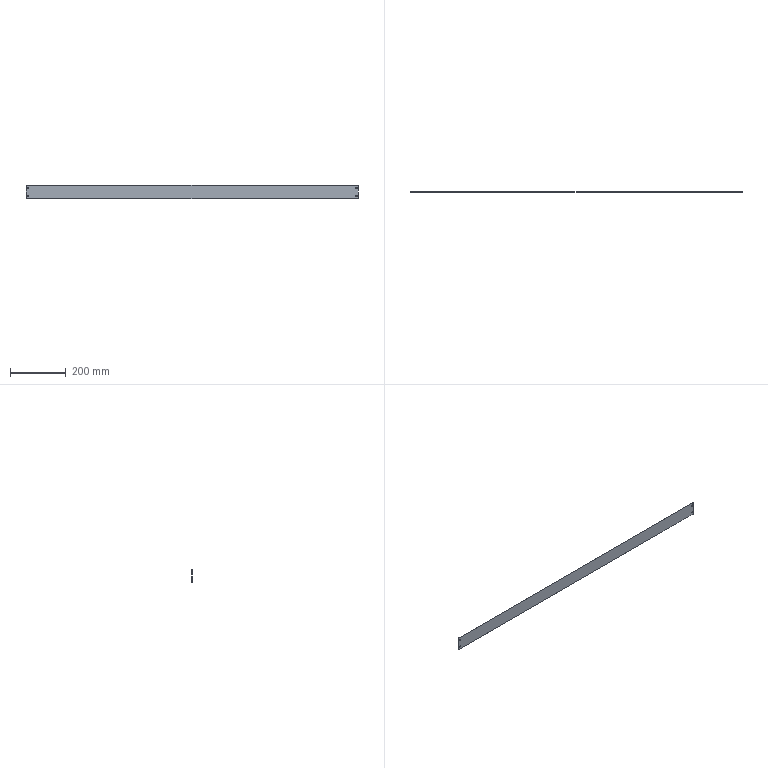Part | NX | features BREP 1 | 1 solid | 26 faces | box 1190 x 0.2 x 50 mm | volume 11880 mm3 | plane 14 | cylinder 12 | commonest cylinder face diameters 4 x12
STEP:
#1=CARTESIAN_POINT('',(591.,0.2,-16.5));
#2=VERTEX_POINT('',#1);
#3=CARTESIAN_POINT('',(588.,0.2,-16.5));
#4=VERTEX_POINT('',#3);
#5=CARTESIAN_POINT('',(591.,0.2,-16.5));
#6=DIRECTION('',(-1.,0.,0.));
#7=VECTOR('',#6,1000.);
#8=LINE('',#5,#7);
#9=EDGE_CURVE('',#2,#4,#8,.T.);
#10=ORIENTED_EDGE('',*,*,#9,.T.);
#11=CARTESIAN_POINT('',(588.,0.,-16.5));
#12=VERTEX_POINT('',#11);
#13=CARTESIAN_POINT('',(588.,0.,-16.5));
#14=DIRECTION('',(0.,1.,0.));
#15=VECTOR('',#14,1000.);
#16=LINE('',#13,#15);
#17=EDGE_CURVE('',#12,#4,#16,.T.);
#18=ORIENTED_EDGE('',*,*,#17,.F.);
#19=CARTESIAN_POINT('',(591.,0.,-16.5));
#20=VERTEX_POINT('',#19);
#21=CARTESIAN_POINT('',(591.,0.,-16.5));
#22=DIRECTION('',(-1.,0.,0.));
#23=VECTOR('',#22,1000.);
#24=LINE('',#21,#23);
#25=EDGE_CURVE('',#20,#12,#24,.T.);
#26=ORIENTED_EDGE('',*,*,#25,.F.);
#27=CARTESIAN_POINT('',(591.,0.,-16.5));
#28=DIRECTION('',(0.,1.,0.));
#29=VECTOR('',#28,1000.);
#30=LINE('',#27,#29);
#31=EDGE_CURVE('',#20,#2,#30,.T.);
#32=ORIENTED_EDGE('',*,*,#31,.T.);
#33=EDGE_LOOP('',(#10,#18,#26,#32));
#34=FACE_BOUND('',#33,.T.);
#35=CARTESIAN_POINT('',(591.,0.,-16.5));
#36=DIRECTION('',(0.,0.,-1.));
#37=DIRECTION('',(-1.,0.,0.));
#38=AXIS2_PLACEMENT_3D('',#35,#36,#37);
#39=PLANE('',#38);
#40=ADVANCED_FACE('',(#34),#39,.F.);
#41=CARTESIAN_POINT('',(588.,0.2,-12.5));
#42=VERTEX_POINT('',#41);
#43=CARTESIAN_POINT('',(588.,0.2,-14.5));
#44=DIRECTION('',(0.,1.,0.));
#45=DIRECTION('',(0.,0.,-1.));
#46=AXIS2_PLACEMENT_3D('',#43,#44,#45);
#47=CIRCLE('',#46,2.);
#48=EDGE_CURVE('',#4,#42,#47,.T.);
#49=ORIENTED_EDGE('',*,*,#48,.T.);
#50=CARTESIAN_POINT('',(588.,0.,-12.5));
#51=VERTEX_POINT('',#50);
#52=CARTESIAN_POINT('',(588.,0.,-12.5));
#53=DIRECTION('',(0.,1.,0.));
#54=VECTOR('',#53,1000.);
#55=LINE('',#52,#54);
#56=EDGE_CURVE('',#51,#42,#55,.T.);
#57=ORIENTED_EDGE('',*,*,#56,.F.);
#58=CARTESIAN_POINT('',(588.,0.,-14.5));
#59=DIRECTION('',(0.,1.,0.));
#60=DIRECTION('',(0.,0.,-1.));
#61=AXIS2_PLACEMENT_3D('',#58,#59,#60);
#62=CIRCLE('',#61,2.);
#63=EDGE_CURVE('',#12,#51,#62,.T.);
#64=ORIENTED_EDGE('',*,*,#63,.F.);
#65=ORIENTED_EDGE('',*,*,#17,.T.);
#66=EDGE_LOOP('',(#49,#57,#64,#65));
#67=FACE_BOUND('',#66,.T.);
#68=CARTESIAN_POINT('',(588.,0.,-14.5));
#69=DIRECTION('',(0.,1.,0.));
#70=DIRECTION('',(0.,0.,1.));
#71=AXIS2_PLACEMENT_3D('',#68,#69,#70);
#72=CYLINDRICAL_SURFACE('',#71,2.);
#73=ADVANCED_FACE('',(#67),#72,.F.);
#74=CARTESIAN_POINT('',(591.,0.2,-12.5));
#75=VERTEX_POINT('',#74);
#76=CARTESIAN_POINT('',(591.,0.2,-12.5));
#77=DIRECTION('',(1.,0.,0.));
#78=VECTOR('',#77,1000.);
#79=LINE('',#76,#78);
#80=EDGE_CURVE('',#42,#75,#79,.T.);
#81=ORIENTED_EDGE('',*,*,#80,.T.);
#82=CARTESIAN_POINT('',(591.,0.,-12.5));
#83=VERTEX_POINT('',#82);
#84=CARTESIAN_POINT('',(591.,0.,-12.5));
#85=DIRECTION('',(0.,1.,0.));
#86=VECTOR('',#85,1000.);
#87=LINE('',#84,#86);
#88=EDGE_CURVE('',#83,#75,#87,.T.);
#89=ORIENTED_EDGE('',*,*,#88,.F.);
#90=CARTESIAN_POINT('',(591.,0.,-12.5));
#91=DIRECTION('',(1.,0.,0.));
#92=VECTOR('',#91,1000.);
#93=LINE('',#90,#92);
#94=EDGE_CURVE('',#51,#83,#93,.T.);
#95=ORIENTED_EDGE('',*,*,#94,.F.);
#96=ORIENTED_EDGE('',*,*,#56,.T.);
#97=EDGE_LOOP('',(#81,#89,#95,#96));
#98=FACE_BOUND('',#97,.T.);
#99=CARTESIAN_POINT('',(591.,0.,-12.5));
#100=DIRECTION('',(0.,0.,1.));
#101=DIRECTION('',(1.,0.,0.));
#102=AXIS2_PLACEMENT_3D('',#99,#100,#101);
#103=PLANE('',#102);
#104=ADVANCED_FACE('',(#98),#103,.F.);
#105=CARTESIAN_POINT('',(591.,0.2,-14.5));
#106=DIRECTION('',(0.,1.,0.));
#107=DIRECTION('',(0.,0.,-1.));
#108=AXIS2_PLACEMENT_3D('',#105,#106,#107);
#109=CIRCLE('',#108,2.);
#110=EDGE_CURVE('',#75,#2,#109,.T.);
#111=ORIENTED_EDGE('',*,*,#110,.T.);
#112=ORIENTED_EDGE('',*,*,#31,.F.);
#113=CARTESIAN_POINT('',(591.,0.,-14.5));
#114=DIRECTION('',(0.,1.,0.));
#115=DIRECTION('',(0.,0.,-1.));
#116=AXIS2_PLACEMENT_3D('',#113,#114,#115);
#117=CIRCLE('',#116,2.);
#118=EDGE_CURVE('',#83,#20,#117,.T.);
#119=ORIENTED_EDGE('',*,*,#118,.F.);
#120=ORIENTED_EDGE('',*,*,#88,.T.);
#121=EDGE_LOOP('',(#111,#112,#119,#120));
#122=FACE_BOUND('',#121,.T.);
#123=CARTESIAN_POINT('',(591.,0.,-14.5));
#124=DIRECTION('',(0.,1.,0.));
#125=DIRECTION('',(0.,0.,1.));
#126=AXIS2_PLACEMENT_3D('',#123,#124,#125);
#127=CYLINDRICAL_SURFACE('',#126,2.);
#128=ADVANCED_FACE('',(#122),#127,.F.);
#129=CARTESIAN_POINT('',(591.,0.2,12.5));
#130=VERTEX_POINT('',#129);
#131=CARTESIAN_POINT('',(588.,0.2,12.5));
#132=VERTEX_POINT('',#131);
#133=CARTESIAN_POINT('',(591.,0.2,12.5));
#134=DIRECTION('',(-1.,0.,0.));
#135=VECTOR('',#134,1000.);
#136=LINE('',#133,#135);
#137=EDGE_CURVE('',#130,#132,#136,.T.);
#138=ORIENTED_EDGE('',*,*,#137,.T.);
#139=CARTESIAN_POINT('',(588.,0.,12.5));
#140=VERTEX_POINT('',#139);
#141=CARTESIAN_POINT('',(588.,0.,12.5));
#142=DIRECTION('',(0.,1.,0.));
#143=VECTOR('',#142,1000.);
#144=LINE('',#141,#143);
#145=EDGE_CURVE('',#140,#132,#144,.T.);
#146=ORIENTED_EDGE('',*,*,#145,.F.);
#147=CARTESIAN_POINT('',(591.,0.,12.5));
#148=VERTEX_POINT('',#147);
#149=CARTESIAN_POINT('',(591.,0.,12.5));
#150=DIRECTION('',(-1.,0.,0.));
#151=VECTOR('',#150,1000.);
#152=LINE('',#149,#151);
#153=EDGE_CURVE('',#148,#140,#152,.T.);
#154=ORIENTED_EDGE('',*,*,#153,.F.);
#155=CARTESIAN_POINT('',(591.,0.,12.5));
#156=DIRECTION('',(0.,1.,0.));
#157=VECTOR('',#156,1000.);
#158=LINE('',#155,#157);
#159=EDGE_CURVE('',#148,#130,#158,.T.);
#160=ORIENTED_EDGE('',*,*,#159,.T.);
#161=EDGE_LOOP('',(#138,#146,#154,#160));
#162=FACE_BOUND('',#161,.T.);
#163=CARTESIAN_POINT('',(591.,0.,12.5));
#164=DIRECTION('',(0.,0.,-1.));
#165=DIRECTION('',(-1.,0.,0.));
#166=AXIS2_PLACEMENT_3D('',#163,#164,#165);
#167=PLANE('',#166);
#168=ADVANCED_FACE('',(#162),#167,.F.);
#169=CARTESIAN_POINT('',(588.,0.2,16.5));
#170=VERTEX_POINT('',#169);
#171=CARTESIAN_POINT('',(588.,0.2,14.5));
#172=DIRECTION('',(0.,1.,0.));
#173=DIRECTION('',(0.,0.,-1.));
#174=AXIS2_PLACEMENT_3D('',#171,#172,#173);
#175=CIRCLE('',#174,2.);
#176=EDGE_CURVE('',#132,#170,#175,.T.);
#177=ORIENTED_EDGE('',*,*,#176,.T.);
#178=CARTESIAN_POINT('',(588.,0.,16.5));
#179=VERTEX_POINT('',#178);
#180=CARTESIAN_POINT('',(588.,0.,16.5));
#181=DIRECTION('',(0.,1.,0.));
#182=VECTOR('',#181,1000.);
#183=LINE('',#180,#182);
#184=EDGE_CURVE('',#179,#170,#183,.T.);
#185=ORIENTED_EDGE('',*,*,#184,.F.);
#186=CARTESIAN_POINT('',(588.,0.,14.5));
#187=DIRECTION('',(0.,1.,0.));
#188=DIRECTION('',(0.,0.,-1.));
#189=AXIS2_PLACEMENT_3D('',#186,#187,#188);
#190=CIRCLE('',#189,2.);
#191=EDGE_CURVE('',#140,#179,#190,.T.);
#192=ORIENTED_EDGE('',*,*,#191,.F.);
#193=ORIENTED_EDGE('',*,*,#145,.T.);
#194=EDGE_LOOP('',(#177,#185,#192,#193));
#195=FACE_BOUND('',#194,.T.);
#196=CARTESIAN_POINT('',(588.,0.,14.5));
#197=DIRECTION('',(0.,1.,0.));
#198=DIRECTION('',(0.,0.,1.));
#199=AXIS2_PLACEMENT_3D('',#196,#197,#198);
#200=CYLINDRICAL_SURFACE('',#199,2.);
#201=ADVANCED_FACE('',(#195),#200,.F.);
#202=CARTESIAN_POINT('',(591.,0.2,16.5));
#203=VERTEX_POINT('',#202);
#204=CARTESIAN_POINT('',(591.,0.2,16.5));
#205=DIRECTION('',(1.,0.,0.));
#206=VECTOR('',#205,1000.);
#207=LINE('',#204,#206);
#208=EDGE_CURVE('',#170,#203,#207,.T.);
#209=ORIENTED_EDGE('',*,*,#208,.T.);
#210=CARTESIAN_POINT('',(591.,0.,16.5));
#211=VERTEX_POINT('',#210);
#212=CARTESIAN_POINT('',(591.,0.,16.5));
#213=DIRECTION('',(0.,1.,0.));
#214=VECTOR('',#213,1000.);
#215=LINE('',#212,#214);
#216=EDGE_CURVE('',#211,#203,#215,.T.);
#217=ORIENTED_EDGE('',*,*,#216,.F.);
#218=CARTESIAN_POINT('',(591.,0.,16.5));
#219=DIRECTION('',(1.,0.,0.));
#220=VECTOR('',#219,1000.);
#221=LINE('',#218,#220);
#222=EDGE_CURVE('',#179,#211,#221,.T.);
#223=ORIENTED_EDGE('',*,*,#222,.F.);
#224=ORIENTED_EDGE('',*,*,#184,.T.);
#225=EDGE_LOOP('',(#209,#217,#223,#224));
#226=FACE_BOUND('',#225,.T.);
#227=CARTESIAN_POINT('',(591.,0.,16.5));
#228=DIRECTION('',(0.,0.,1.));
#229=DIRECTION('',(1.,0.,0.));
#230=AXIS2_PLACEMENT_3D('',#227,#228,#229);
#231=PLANE('',#230);
#232=ADVANCED_FACE('',(#226),#231,.F.);
#233=CARTESIAN_POINT('',(591.,0.2,14.5));
#234=DIRECTION('',(0.,1.,0.));
#235=DIRECTION('',(0.,0.,-1.));
#236=AXIS2_PLACEMENT_3D('',#233,#234,#235);
#237=CIRCLE('',#236,2.);
#238=EDGE_CURVE('',#203,#130,#237,.T.);
#239=ORIENTED_EDGE('',*,*,#238,.T.);
#240=ORIENTED_EDGE('',*,*,#159,.F.);
#241=CARTESIAN_POINT('',(591.,0.,14.5));
#242=DIRECTION('',(0.,1.,0.));
#243=DIRECTION('',(0.,0.,-1.));
#244=AXIS2_PLACEMENT_3D('',#241,#242,#243);
#245=CIRCLE('',#244,2.);
#246=EDGE_CURVE('',#211,#148,#245,.T.);
#247=ORIENTED_EDGE('',*,*,#246,.F.);
#248=ORIENTED_EDGE('',*,*,#216,.T.);
#249=EDGE_LOOP('',(#239,#240,#247,#248));
#250=FACE_BOUND('',#249,.T.);
#251=CARTESIAN_POINT('',(591.,0.,14.5));
#252=DIRECTION('',(0.,1.,0.));
#253=DIRECTION('',(0.,0.,1.));
#254=AXIS2_PLACEMENT_3D('',#251,#252,#253);
#255=CYLINDRICAL_SURFACE('',#254,2.);
#256=ADVANCED_FACE('',(#250),#255,.F.);
#257=CARTESIAN_POINT('',(-591.,0.2,16.5));
#258=VERTEX_POINT('',#257);
#259=CARTESIAN_POINT('',(-588.,0.2,16.5));
#260=VERTEX_POINT('',#259);
#261=CARTESIAN_POINT('',(-591.,0.2,16.5));
#262=DIRECTION('',(1.,0.,0.));
#263=VECTOR('',#262,1000.);
#264=LINE('',#261,#263);
#265=EDGE_CURVE('',#258,#260,#264,.T.);
#266=ORIENTED_EDGE('',*,*,#265,.T.);
#267=CARTESIAN_POINT('',(-588.,0.,16.5));
#268=VERTEX_POINT('',#267);
#269=CARTESIAN_POINT('',(-588.,0.,16.5));
#270=DIRECTION('',(0.,1.,0.));
#271=VECTOR('',#270,1000.);
#272=LINE('',#269,#271);
#273=EDGE_CURVE('',#268,#260,#272,.T.);
#274=ORIENTED_EDGE('',*,*,#273,.F.);
#275=CARTESIAN_POINT('',(-591.,0.,16.5));
#276=VERTEX_POINT('',#275);
#277=CARTESIAN_POINT('',(-591.,0.,16.5));
#278=DIRECTION('',(1.,0.,0.));
#279=VECTOR('',#278,1000.);
#280=LINE('',#277,#279);
#281=EDGE_CURVE('',#276,#268,#280,.T.);
#282=ORIENTED_EDGE('',*,*,#281,.F.);
#283=CARTESIAN_POINT('',(-591.,0.,16.5));
#284=DIRECTION('',(0.,1.,0.));
#285=VECTOR('',#284,1000.);
#286=LINE('',#283,#285);
#287=EDGE_CURVE('',#276,#258,#286,.T.);
#288=ORIENTED_EDGE('',*,*,#287,.T.);
#289=EDGE_LOOP('',(#266,#274,#282,#288));
#290=FACE_BOUND('',#289,.T.);
#291=CARTESIAN_POINT('',(-591.,0.,16.5));
#292=DIRECTION('',(0.,0.,1.));
#293=DIRECTION('',(1.,0.,0.));
#294=AXIS2_PLACEMENT_3D('',#291,#292,#293);
#295=PLANE('',#294);
#296=ADVANCED_FACE('',(#290),#295,.F.);
#297=CARTESIAN_POINT('',(-588.,0.2,12.5));
#298=VERTEX_POINT('',#297);
#299=CARTESIAN_POINT('',(-588.,0.2,14.5));
#300=DIRECTION('',(0.,1.,0.));
#301=DIRECTION('',(0.,0.,1.));
#302=AXIS2_PLACEMENT_3D('',#299,#300,#301);
#303=CIRCLE('',#302,2.);
#304=EDGE_CURVE('',#260,#298,#303,.T.);
#305=ORIENTED_EDGE('',*,*,#304,.T.);
#306=CARTESIAN_POINT('',(-588.,0.,12.5));
#307=VERTEX_POINT('',#306);
#308=CARTESIAN_POINT('',(-588.,0.,12.5));
#309=DIRECTION('',(0.,1.,0.));
#310=VECTOR('',#309,1000.);
#311=LINE('',#308,#310);
#312=EDGE_CURVE('',#307,#298,#311,.T.);
#313=ORIENTED_EDGE('',*,*,#312,.F.);
#314=CARTESIAN_POINT('',(-588.,0.,14.5));
#315=DIRECTION('',(0.,1.,0.));
#316=DIRECTION('',(0.,0.,1.));
#317=AXIS2_PLACEMENT_3D('',#314,#315,#316);
#318=CIRCLE('',#317,2.);
#319=EDGE_CURVE('',#268,#307,#318,.T.);
#320=ORIENTED_EDGE('',*,*,#319,.F.);
#321=ORIENTED_EDGE('',*,*,#273,.T.);
#322=EDGE_LOOP('',(#305,#313,#320,#321));
#323=FACE_BOUND('',#322,.T.);
#324=CARTESIAN_POINT('',(-588.,0.,14.5));
#325=DIRECTION('',(0.,1.,0.));
#326=DIRECTION('',(0.,0.,1.));
#327=AXIS2_PLACEMENT_3D('',#324,#325,#326);
#328=CYLINDRICAL_SURFACE('',#327,2.);
#329=ADVANCED_FACE('',(#323),#328,.F.);
#330=CARTESIAN_POINT('',(-591.,0.2,12.5));
#331=VERTEX_POINT('',#330);
#332=CARTESIAN_POINT('',(-591.,0.2,12.5));
#333=DIRECTION('',(-1.,0.,0.));
#334=VECTOR('',#333,1000.);
#335=LINE('',#332,#334);
#336=EDGE_CURVE('',#298,#331,#335,.T.);
#337=ORIENTED_EDGE('',*,*,#336,.T.);
#338=CARTESIAN_POINT('',(-591.,0.,12.5));
#339=VERTEX_POINT('',#338);
#340=CARTESIAN_POINT('',(-591.,0.,12.5));
#341=DIRECTION('',(0.,1.,0.));
#342=VECTOR('',#341,1000.);
#343=LINE('',#340,#342);
#344=EDGE_CURVE('',#339,#331,#343,.T.);
#345=ORIENTED_EDGE('',*,*,#344,.F.);
#346=CARTESIAN_POINT('',(-591.,0.,12.5));
#347=DIRECTION('',(-1.,0.,0.));
#348=VECTOR('',#347,1000.);
#349=LINE('',#346,#348);
#350=EDGE_CURVE('',#307,#339,#349,.T.);
#351=ORIENTED_EDGE('',*,*,#350,.F.);
#352=ORIENTED_EDGE('',*,*,#312,.T.);
#353=EDGE_LOOP('',(#337,#345,#351,#352));
#354=FACE_BOUND('',#353,.T.);
#355=CARTESIAN_POINT('',(-591.,0.,12.5));
#356=DIRECTION('',(0.,0.,-1.));
#357=DIRECTION('',(-1.,0.,0.));
#358=AXIS2_PLACEMENT_3D('',#355,#356,#357);
#359=PLANE('',#358);
#360=ADVANCED_FACE('',(#354),#359,.F.);
#361=CARTESIAN_POINT('',(-591.,0.2,14.5));
#362=DIRECTION('',(0.,1.,0.));
#363=DIRECTION('',(0.,0.,1.));
#364=AXIS2_PLACEMENT_3D('',#361,#362,#363);
#365=CIRCLE('',#364,2.);
#366=EDGE_CURVE('',#331,#258,#365,.T.);
#367=ORIENTED_EDGE('',*,*,#366,.T.);
#368=ORIENTED_EDGE('',*,*,#287,.F.);
#369=CARTESIAN_POINT('',(-591.,0.,14.5));
#370=DIRECTION('',(0.,1.,0.));
#371=DIRECTION('',(0.,0.,1.));
#372=AXIS2_PLACEMENT_3D('',#369,#370,#371);
#373=CIRCLE('',#372,2.);
#374=EDGE_CURVE('',#339,#276,#373,.T.);
#375=ORIENTED_EDGE('',*,*,#374,.F.);
#376=ORIENTED_EDGE('',*,*,#344,.T.);
#377=EDGE_LOOP('',(#367,#368,#375,#376));
#378=FACE_BOUND('',#377,.T.);
#379=CARTESIAN_POINT('',(-591.,0.,14.5));
#380=DIRECTION('',(0.,1.,0.));
#381=DIRECTION('',(0.,0.,1.));
#382=AXIS2_PLACEMENT_3D('',#379,#380,#381);
#383=CYLINDRICAL_SURFACE('',#382,2.);
#384=ADVANCED_FACE('',(#378),#383,.F.);
#385=CARTESIAN_POINT('',(-591.,0.2,-12.5));
#386=VERTEX_POINT('',#385);
#387=CARTESIAN_POINT('',(-588.,0.2,-12.5));
#388=VERTEX_POINT('',#387);
#389=CARTESIAN_POINT('',(-591.,0.2,-12.5));
#390=DIRECTION('',(1.,0.,0.));
#391=VECTOR('',#390,1000.);
#392=LINE('',#389,#391);
#393=EDGE_CURVE('',#386,#388,#392,.T.);
#394=ORIENTED_EDGE('',*,*,#393,.T.);
#395=CARTESIAN_POINT('',(-588.,0.,-12.5));
#396=VERTEX_POINT('',#395);
#397=CARTESIAN_POINT('',(-588.,0.,-12.5));
#398=DIRECTION('',(0.,1.,0.));
#399=VECTOR('',#398,1000.);
#400=LINE('',#397,#399);
#401=EDGE_CURVE('',#396,#388,#400,.T.);
#402=ORIENTED_EDGE('',*,*,#401,.F.);
#403=CARTESIAN_POINT('',(-591.,0.,-12.5));
#404=VERTEX_POINT('',#403);
#405=CARTESIAN_POINT('',(-591.,0.,-12.5));
#406=DIRECTION('',(1.,0.,0.));
#407=VECTOR('',#406,1000.);
#408=LINE('',#405,#407);
#409=EDGE_CURVE('',#404,#396,#408,.T.);
#410=ORIENTED_EDGE('',*,*,#409,.F.);
#411=CARTESIAN_POINT('',(-591.,0.,-12.5));
#412=DIRECTION('',(0.,1.,0.));
#413=VECTOR('',#412,1000.);
#414=LINE('',#411,#413);
#415=EDGE_CURVE('',#404,#386,#414,.T.);
#416=ORIENTED_EDGE('',*,*,#415,.T.);
#417=EDGE_LOOP('',(#394,#402,#410,#416));
#418=FACE_BOUND('',#417,.T.);
#419=CARTESIAN_POINT('',(-591.,0.,-12.5));
#420=DIRECTION('',(0.,0.,1.));
#421=DIRECTION('',(1.,0.,0.));
#422=AXIS2_PLACEMENT_3D('',#419,#420,#421);
#423=PLANE('',#422);
#424=ADVANCED_FACE('',(#418),#423,.F.);
#425=CARTESIAN_POINT('',(-588.,0.2,-16.5));
#426=VERTEX_POINT('',#425);
#427=CARTESIAN_POINT('',(-588.,0.2,-14.5));
#428=DIRECTION('',(0.,1.,0.));
#429=DIRECTION('',(0.,0.,1.));
#430=AXIS2_PLACEMENT_3D('',#427,#428,#429);
#431=CIRCLE('',#430,2.);
#432=EDGE_CURVE('',#388,#426,#431,.T.);
#433=ORIENTED_EDGE('',*,*,#432,.T.);
#434=CARTESIAN_POINT('',(-588.,0.,-16.5));
#435=VERTEX_POINT('',#434);
#436=CARTESIAN_POINT('',(-588.,0.,-16.5));
#437=DIRECTION('',(0.,1.,0.));
#438=VECTOR('',#437,1000.);
#439=LINE('',#436,#438);
#440=EDGE_CURVE('',#435,#426,#439,.T.);
#441=ORIENTED_EDGE('',*,*,#440,.F.);
#442=CARTESIAN_POINT('',(-588.,0.,-14.5));
#443=DIRECTION('',(0.,1.,0.));
#444=DIRECTION('',(0.,0.,1.));
#445=AXIS2_PLACEMENT_3D('',#442,#443,#444);
#446=CIRCLE('',#445,2.);
#447=EDGE_CURVE('',#396,#435,#446,.T.);
#448=ORIENTED_EDGE('',*,*,#447,.F.);
#449=ORIENTED_EDGE('',*,*,#401,.T.);
#450=EDGE_LOOP('',(#433,#441,#448,#449));
#451=FACE_BOUND('',#450,.T.);
#452=CARTESIAN_POINT('',(-588.,0.,-14.5));
#453=DIRECTION('',(0.,1.,0.));
#454=DIRECTION('',(0.,0.,1.));
#455=AXIS2_PLACEMENT_3D('',#452,#453,#454);
#456=CYLINDRICAL_SURFACE('',#455,2.);
#457=ADVANCED_FACE('',(#451),#456,.F.);
#458=CARTESIAN_POINT('',(-591.,0.2,-16.5));
#459=VERTEX_POINT('',#458);
#460=CARTESIAN_POINT('',(-591.,0.2,-16.5));
#461=DIRECTION('',(-1.,0.,0.));
#462=VECTOR('',#461,1000.);
#463=LINE('',#460,#462);
#464=EDGE_CURVE('',#426,#459,#463,.T.);
#465=ORIENTED_EDGE('',*,*,#464,.T.);
#466=CARTESIAN_POINT('',(-591.,0.,-16.5));
#467=VERTEX_POINT('',#466);
#468=CARTESIAN_POINT('',(-591.,0.,-16.5));
#469=DIRECTION('',(0.,1.,0.));
#470=VECTOR('',#469,1000.);
#471=LINE('',#468,#470);
#472=EDGE_CURVE('',#467,#459,#471,.T.);
#473=ORIENTED_EDGE('',*,*,#472,.F.);
#474=CARTESIAN_POINT('',(-591.,0.,-16.5));
#475=DIRECTION('',(-1.,0.,0.));
#476=VECTOR('',#475,1000.);
#477=LINE('',#474,#476);
#478=EDGE_CURVE('',#435,#467,#477,.T.);
#479=ORIENTED_EDGE('',*,*,#478,.F.);
#480=ORIENTED_EDGE('',*,*,#440,.T.);
#481=EDGE_LOOP('',(#465,#473,#479,#480));
#482=FACE_BOUND('',#481,.T.);
#483=CARTESIAN_POINT('',(-591.,0.,-16.5));
#484=DIRECTION('',(0.,0.,-1.));
#485=DIRECTION('',(-1.,0.,0.));
#486=AXIS2_PLACEMENT_3D('',#483,#484,#485);
#487=PLANE('',#486);
#488=ADVANCED_FACE('',(#482),#487,.F.);
#489=CARTESIAN_POINT('',(-591.,0.2,-14.5));
#490=DIRECTION('',(0.,1.,0.));
#491=DIRECTION('',(0.,0.,1.));
#492=AXIS2_PLACEMENT_3D('',#489,#490,#491);
#493=CIRCLE('',#492,2.);
#494=EDGE_CURVE('',#459,#386,#493,.T.);
#495=ORIENTED_EDGE('',*,*,#494,.T.);
#496=ORIENTED_EDGE('',*,*,#415,.F.);
#497=CARTESIAN_POINT('',(-591.,0.,-14.5));
#498=DIRECTION('',(0.,1.,0.));
#499=DIRECTION('',(0.,0.,1.));
#500=AXIS2_PLACEMENT_3D('',#497,#498,#499);
#501=CIRCLE('',#500,2.);
#502=EDGE_CURVE('',#467,#404,#501,.T.);
#503=ORIENTED_EDGE('',*,*,#502,.F.);
#504=ORIENTED_EDGE('',*,*,#472,.T.);
#505=EDGE_LOOP('',(#495,#496,#503,#504));
#506=FACE_BOUND('',#505,.T.);
#507=CARTESIAN_POINT('',(-591.,0.,-14.5));
#508=DIRECTION('',(0.,1.,0.));
#509=DIRECTION('',(0.,0.,1.));
#510=AXIS2_PLACEMENT_3D('',#507,#508,#509);
#511=CYLINDRICAL_SURFACE('',#510,2.);
#512=ADVANCED_FACE('',(#506),#511,.F.);
#513=CARTESIAN_POINT('',(595.,0.,-23.));
#514=VERTEX_POINT('',#513);
#515=CARTESIAN_POINT('',(593.,0.,-25.));
#516=VERTEX_POINT('',#515);
#517=CARTESIAN_POINT('',(593.,0.,-23.));
#518=DIRECTION('',(0.,1.,0.));
#519=DIRECTION('',(0.,0.,-1.));
#520=AXIS2_PLACEMENT_3D('',#517,#518,#519);
#521=CIRCLE('',#520,2.);
#522=EDGE_CURVE('',#514,#516,#521,.T.);
#523=ORIENTED_EDGE('',*,*,#522,.F.);
#524=CARTESIAN_POINT('',(595.,0.,23.));
#525=VERTEX_POINT('',#524);
#526=CARTESIAN_POINT('',(595.,0.,23.));
#527=DIRECTION('',(0.,0.,-1.));
#528=VECTOR('',#527,1000.);
#529=LINE('',#526,#528);
#530=EDGE_CURVE('',#525,#514,#529,.T.);
#531=ORIENTED_EDGE('',*,*,#530,.F.);
#532=CARTESIAN_POINT('',(593.,0.,25.));
#533=VERTEX_POINT('',#532);
#534=CARTESIAN_POINT('',(593.,0.,23.));
#535=DIRECTION('',(0.,1.,0.));
#536=DIRECTION('',(0.,0.,1.));
#537=AXIS2_PLACEMENT_3D('',#534,#535,#536);
#538=CIRCLE('',#537,2.);
#539=EDGE_CURVE('',#533,#525,#538,.T.);
#540=ORIENTED_EDGE('',*,*,#539,.F.);
#541=CARTESIAN_POINT('',(-593.,0.,25.));
#542=VERTEX_POINT('',#541);
#543=CARTESIAN_POINT('',(-593.,0.,25.));
#544=DIRECTION('',(1.,0.,0.));
#545=VECTOR('',#544,1000.);
#546=LINE('',#543,#545);
#547=EDGE_CURVE('',#542,#533,#546,.T.);
#548=ORIENTED_EDGE('',*,*,#547,.F.);
#549=CARTESIAN_POINT('',(-595.,0.,23.));
#550=VERTEX_POINT('',#549);
#551=CARTESIAN_POINT('',(-593.,0.,23.));
#552=DIRECTION('',(0.,1.,0.));
#553=DIRECTION('',(0.,0.,-1.));
#554=AXIS2_PLACEMENT_3D('',#551,#552,#553);
#555=CIRCLE('',#554,2.);
#556=EDGE_CURVE('',#550,#542,#555,.T.);
#557=ORIENTED_EDGE('',*,*,#556,.F.);
#558=CARTESIAN_POINT('',(-595.,0.,-23.));
#559=VERTEX_POINT('',#558);
#560=CARTESIAN_POINT('',(-595.,0.,23.));
#561=DIRECTION('',(0.,0.,1.));
#562=VECTOR('',#561,1000.);
#563=LINE('',#560,#562);
#564=EDGE_CURVE('',#559,#550,#563,.T.);
#565=ORIENTED_EDGE('',*,*,#564,.F.);
#566=CARTESIAN_POINT('',(-593.,0.,-25.));
#567=VERTEX_POINT('',#566);
#568=CARTESIAN_POINT('',(-593.,0.,-23.));
#569=DIRECTION('',(0.,1.,0.));
#570=DIRECTION('',(0.,0.,-1.));
#571=AXIS2_PLACEMENT_3D('',#568,#569,#570);
#572=CIRCLE('',#571,2.);
#573=EDGE_CURVE('',#567,#559,#572,.T.);
#574=ORIENTED_EDGE('',*,*,#573,.F.);
#575=CARTESIAN_POINT('',(-593.,0.,-25.));
#576=DIRECTION('',(-1.,0.,0.));
#577=VECTOR('',#576,1000.);
#578=LINE('',#575,#577);
#579=EDGE_CURVE('',#516,#567,#578,.T.);
#580=ORIENTED_EDGE('',*,*,#579,.F.);
#581=EDGE_LOOP('',(#523,#531,#540,#548,#557,#565,#574,#580));
#582=FACE_BOUND('',#581,.T.);
#583=ORIENTED_EDGE('',*,*,#502,.T.);
#584=ORIENTED_EDGE('',*,*,#409,.T.);
#585=ORIENTED_EDGE('',*,*,#447,.T.);
#586=ORIENTED_EDGE('',*,*,#478,.T.);
#587=EDGE_LOOP('',(#583,#584,#585,#586));
#588=FACE_BOUND('',#587,.T.);
#589=ORIENTED_EDGE('',*,*,#374,.T.);
#590=ORIENTED_EDGE('',*,*,#281,.T.);
#591=ORIENTED_EDGE('',*,*,#319,.T.);
#592=ORIENTED_EDGE('',*,*,#350,.T.);
#593=EDGE_LOOP('',(#589,#590,#591,#592));
#594=FACE_BOUND('',#593,.T.);
#595=ORIENTED_EDGE('',*,*,#246,.T.);
#596=ORIENTED_EDGE('',*,*,#153,.T.);
#597=ORIENTED_EDGE('',*,*,#191,.T.);
#598=ORIENTED_EDGE('',*,*,#222,.T.);
#599=EDGE_LOOP('',(#595,#596,#597,#598));
#600=FACE_BOUND('',#599,.T.);
#601=ORIENTED_EDGE('',*,*,#118,.T.);
#602=ORIENTED_EDGE('',*,*,#25,.T.);
#603=ORIENTED_EDGE('',*,*,#63,.T.);
#604=ORIENTED_EDGE('',*,*,#94,.T.);
#605=EDGE_LOOP('',(#601,#602,#603,#604));
#606=FACE_BOUND('',#605,.T.);
#607=CARTESIAN_POINT('',(593.,0.,-23.));
#608=DIRECTION('',(0.,-1.,0.));
#609=DIRECTION('',(0.,0.,-1.));
#610=AXIS2_PLACEMENT_3D('',#607,#608,#609);
#611=PLANE('',#610);
#612=ADVANCED_FACE('',(#582,#588,#594,#600,#606),#611,.T.);
#613=CARTESIAN_POINT('',(595.,0.2,-23.));
#614=VERTEX_POINT('',#613);
#615=CARTESIAN_POINT('',(593.,0.2,-25.));
#616=VERTEX_POINT('',#615);
#617=CARTESIAN_POINT('',(593.,0.2,-23.));
#618=DIRECTION('',(0.,1.,0.));
#619=DIRECTION('',(0.,0.,-1.));
#620=AXIS2_PLACEMENT_3D('',#617,#618,#619);
#621=CIRCLE('',#620,2.);
#622=EDGE_CURVE('',#614,#616,#621,.T.);
#623=ORIENTED_EDGE('',*,*,#622,.T.);
#624=CARTESIAN_POINT('',(-593.,0.2,-25.));
#625=VERTEX_POINT('',#624);
#626=CARTESIAN_POINT('',(-593.,0.2,-25.));
#627=DIRECTION('',(-1.,0.,0.));
#628=VECTOR('',#627,1000.);
#629=LINE('',#626,#628);
#630=EDGE_CURVE('',#616,#625,#629,.T.);
#631=ORIENTED_EDGE('',*,*,#630,.T.);
#632=CARTESIAN_POINT('',(-595.,0.2,-23.));
#633=VERTEX_POINT('',#632);
#634=CARTESIAN_POINT('',(-593.,0.2,-23.));
#635=DIRECTION('',(0.,1.,0.));
#636=DIRECTION('',(0.,0.,-1.));
#637=AXIS2_PLACEMENT_3D('',#634,#635,#636);
#638=CIRCLE('',#637,2.);
#639=EDGE_CURVE('',#625,#633,#638,.T.);
#640=ORIENTED_EDGE('',*,*,#639,.T.);
#641=CARTESIAN_POINT('',(-595.,0.2,23.));
#642=VERTEX_POINT('',#641);
#643=CARTESIAN_POINT('',(-595.,0.2,23.));
#644=DIRECTION('',(0.,0.,1.));
#645=VECTOR('',#644,1000.);
#646=LINE('',#643,#645);
#647=EDGE_CURVE('',#633,#642,#646,.T.);
#648=ORIENTED_EDGE('',*,*,#647,.T.);
#649=CARTESIAN_POINT('',(-593.,0.2,25.));
#650=VERTEX_POINT('',#649);
#651=CARTESIAN_POINT('',(-593.,0.2,23.));
#652=DIRECTION('',(0.,1.,0.));
#653=DIRECTION('',(0.,0.,-1.));
#654=AXIS2_PLACEMENT_3D('',#651,#652,#653);
#655=CIRCLE('',#654,2.);
#656=EDGE_CURVE('',#642,#650,#655,.T.);
#657=ORIENTED_EDGE('',*,*,#656,.T.);
#658=CARTESIAN_POINT('',(593.,0.2,25.));
#659=VERTEX_POINT('',#658);
#660=CARTESIAN_POINT('',(-593.,0.2,25.));
#661=DIRECTION('',(1.,0.,0.));
#662=VECTOR('',#661,1000.);
#663=LINE('',#660,#662);
#664=EDGE_CURVE('',#650,#659,#663,.T.);
#665=ORIENTED_EDGE('',*,*,#664,.T.);
#666=CARTESIAN_POINT('',(595.,0.2,23.));
#667=VERTEX_POINT('',#666);
#668=CARTESIAN_POINT('',(593.,0.2,23.));
#669=DIRECTION('',(0.,1.,0.));
#670=DIRECTION('',(0.,0.,1.));
#671=AXIS2_PLACEMENT_3D('',#668,#669,#670);
#672=CIRCLE('',#671,2.);
#673=EDGE_CURVE('',#659,#667,#672,.T.);
#674=ORIENTED_EDGE('',*,*,#673,.T.);
#675=CARTESIAN_POINT('',(595.,0.2,23.));
#676=DIRECTION('',(0.,0.,-1.));
#677=VECTOR('',#676,1000.);
#678=LINE('',#675,#677);
#679=EDGE_CURVE('',#667,#614,#678,.T.);
#680=ORIENTED_EDGE('',*,*,#679,.T.);
#681=EDGE_LOOP('',(#623,#631,#640,#648,#657,#665,#674,#680));
#682=FACE_BOUND('',#681,.T.);
#683=ORIENTED_EDGE('',*,*,#393,.F.);
#684=ORIENTED_EDGE('',*,*,#494,.F.);
#685=ORIENTED_EDGE('',*,*,#464,.F.);
#686=ORIENTED_EDGE('',*,*,#432,.F.);
#687=EDGE_LOOP('',(#683,#684,#685,#686));
#688=FACE_BOUND('',#687,.T.);
#689=ORIENTED_EDGE('',*,*,#265,.F.);
#690=ORIENTED_EDGE('',*,*,#366,.F.);
#691=ORIENTED_EDGE('',*,*,#336,.F.);
#692=ORIENTED_EDGE('',*,*,#304,.F.);
#693=EDGE_LOOP('',(#689,#690,#691,#692));
#694=FACE_BOUND('',#693,.T.);
#695=ORIENTED_EDGE('',*,*,#137,.F.);
#696=ORIENTED_EDGE('',*,*,#238,.F.);
#697=ORIENTED_EDGE('',*,*,#208,.F.);
#698=ORIENTED_EDGE('',*,*,#176,.F.);
#699=EDGE_LOOP('',(#695,#696,#697,#698));
#700=FACE_BOUND('',#699,.T.);
#701=ORIENTED_EDGE('',*,*,#9,.F.);
#702=ORIENTED_EDGE('',*,*,#110,.F.);
#703=ORIENTED_EDGE('',*,*,#80,.F.);
#704=ORIENTED_EDGE('',*,*,#48,.F.);
#705=EDGE_LOOP('',(#701,#702,#703,#704));
#706=FACE_BOUND('',#705,.T.);
#707=CARTESIAN_POINT('',(593.,0.2,-23.));
#708=DIRECTION('',(0.,-1.,0.));
#709=DIRECTION('',(0.,0.,-1.));
#710=AXIS2_PLACEMENT_3D('',#707,#708,#709);
#711=PLANE('',#710);
#712=ADVANCED_FACE('',(#682,#688,#694,#700,#706),#711,.F.);
#713=ORIENTED_EDGE('',*,*,#530,.T.);
#714=CARTESIAN_POINT('',(595.,0.2,-23.));
#715=DIRECTION('',(0.,-1.,0.));
#716=VECTOR('',#715,1000.);
#717=LINE('',#714,#716);
#718=EDGE_CURVE('',#614,#514,#717,.T.);
#719=ORIENTED_EDGE('',*,*,#718,.F.);
#720=ORIENTED_EDGE('',*,*,#679,.F.);
#721=CARTESIAN_POINT('',(595.,0.2,23.));
#722=DIRECTION('',(0.,-1.,0.));
#723=VECTOR('',#722,1000.);
#724=LINE('',#721,#723);
#725=EDGE_CURVE('',#667,#525,#724,.T.);
#726=ORIENTED_EDGE('',*,*,#725,.T.);
#727=EDGE_LOOP('',(#713,#719,#720,#726));
#728=FACE_BOUND('',#727,.T.);
#729=CARTESIAN_POINT('',(595.,0.2,23.));
#730=DIRECTION('',(-1.,0.,0.));
#731=DIRECTION('',(0.,0.,1.));
#732=AXIS2_PLACEMENT_3D('',#729,#730,#731);
#733=PLANE('',#732);
#734=ADVANCED_FACE('',(#728),#733,.F.);
#735=ORIENTED_EDGE('',*,*,#539,.T.);
#736=ORIENTED_EDGE('',*,*,#725,.F.);
#737=ORIENTED_EDGE('',*,*,#673,.F.);
#738=CARTESIAN_POINT('',(593.,0.2,25.));
#739=DIRECTION('',(0.,-1.,0.));
#740=VECTOR('',#739,1000.);
#741=LINE('',#738,#740);
#742=EDGE_CURVE('',#659,#533,#741,.T.);
#743=ORIENTED_EDGE('',*,*,#742,.T.);
#744=EDGE_LOOP('',(#735,#736,#737,#743));
#745=FACE_BOUND('',#744,.T.);
#746=CARTESIAN_POINT('',(593.,0.2,23.));
#747=DIRECTION('',(0.,-1.,0.));
#748=DIRECTION('',(0.,0.,-1.));
#749=AXIS2_PLACEMENT_3D('',#746,#747,#748);
#750=CYLINDRICAL_SURFACE('',#749,2.);
#751=ADVANCED_FACE('',(#745),#750,.T.);
#752=ORIENTED_EDGE('',*,*,#547,.T.);
#753=ORIENTED_EDGE('',*,*,#742,.F.);
#754=ORIENTED_EDGE('',*,*,#664,.F.);
#755=CARTESIAN_POINT('',(-593.,0.2,25.));
#756=DIRECTION('',(0.,-1.,0.));
#757=VECTOR('',#756,1000.);
#758=LINE('',#755,#757);
#759=EDGE_CURVE('',#650,#542,#758,.T.);
#760=ORIENTED_EDGE('',*,*,#759,.T.);
#761=EDGE_LOOP('',(#752,#753,#754,#760));
#762=FACE_BOUND('',#761,.T.);
#763=CARTESIAN_POINT('',(-593.,0.2,25.));
#764=DIRECTION('',(0.,0.,-1.));
#765=DIRECTION('',(-1.,0.,0.));
#766=AXIS2_PLACEMENT_3D('',#763,#764,#765);
#767=PLANE('',#766);
#768=ADVANCED_FACE('',(#762),#767,.F.);
#769=ORIENTED_EDGE('',*,*,#556,.T.);
#770=ORIENTED_EDGE('',*,*,#759,.F.);
#771=ORIENTED_EDGE('',*,*,#656,.F.);
#772=CARTESIAN_POINT('',(-595.,0.2,23.));
#773=DIRECTION('',(0.,-1.,0.));
#774=VECTOR('',#773,1000.);
#775=LINE('',#772,#774);
#776=EDGE_CURVE('',#642,#550,#775,.T.);
#777=ORIENTED_EDGE('',*,*,#776,.T.);
#778=EDGE_LOOP('',(#769,#770,#771,#777));
#779=FACE_BOUND('',#778,.T.);
#780=CARTESIAN_POINT('',(-593.,0.2,23.));
#781=DIRECTION('',(0.,-1.,0.));
#782=DIRECTION('',(0.,0.,-1.));
#783=AXIS2_PLACEMENT_3D('',#780,#781,#782);
#784=CYLINDRICAL_SURFACE('',#783,2.);
#785=ADVANCED_FACE('',(#779),#784,.T.);
#786=ORIENTED_EDGE('',*,*,#564,.T.);
#787=ORIENTED_EDGE('',*,*,#776,.F.);
#788=ORIENTED_EDGE('',*,*,#647,.F.);
#789=CARTESIAN_POINT('',(-595.,0.2,-23.));
#790=DIRECTION('',(0.,-1.,0.));
#791=VECTOR('',#790,1000.);
#792=LINE('',#789,#791);
#793=EDGE_CURVE('',#633,#559,#792,.T.);
#794=ORIENTED_EDGE('',*,*,#793,.T.);
#795=EDGE_LOOP('',(#786,#787,#788,#794));
#796=FACE_BOUND('',#795,.T.);
#797=CARTESIAN_POINT('',(-595.,0.2,23.));
#798=DIRECTION('',(1.,0.,0.));
#799=DIRECTION('',(0.,0.,-1.));
#800=AXIS2_PLACEMENT_3D('',#797,#798,#799);
#801=PLANE('',#800);
#802=ADVANCED_FACE('',(#796),#801,.F.);
#803=ORIENTED_EDGE('',*,*,#573,.T.);
#804=ORIENTED_EDGE('',*,*,#793,.F.);
#805=ORIENTED_EDGE('',*,*,#639,.F.);
#806=CARTESIAN_POINT('',(-593.,0.2,-25.));
#807=DIRECTION('',(0.,-1.,0.));
#808=VECTOR('',#807,1000.);
#809=LINE('',#806,#808);
#810=EDGE_CURVE('',#625,#567,#809,.T.);
#811=ORIENTED_EDGE('',*,*,#810,.T.);
#812=EDGE_LOOP('',(#803,#804,#805,#811));
#813=FACE_BOUND('',#812,.T.);
#814=CARTESIAN_POINT('',(-593.,0.2,-23.));
#815=DIRECTION('',(0.,-1.,0.));
#816=DIRECTION('',(0.,0.,-1.));
#817=AXIS2_PLACEMENT_3D('',#814,#815,#816);
#818=CYLINDRICAL_SURFACE('',#817,2.);
#819=ADVANCED_FACE('',(#813),#818,.T.);
#820=ORIENTED_EDGE('',*,*,#579,.T.);
#821=ORIENTED_EDGE('',*,*,#810,.F.);
#822=ORIENTED_EDGE('',*,*,#630,.F.);
#823=CARTESIAN_POINT('',(593.,0.2,-25.));
#824=DIRECTION('',(0.,-1.,0.));
#825=VECTOR('',#824,1000.);
#826=LINE('',#823,#825);
#827=EDGE_CURVE('',#616,#516,#826,.T.);
#828=ORIENTED_EDGE('',*,*,#827,.T.);
#829=EDGE_LOOP('',(#820,#821,#822,#828));
#830=FACE_BOUND('',#829,.T.);
#831=CARTESIAN_POINT('',(-593.,0.2,-25.));
#832=DIRECTION('',(0.,0.,1.));
#833=DIRECTION('',(1.,0.,0.));
#834=AXIS2_PLACEMENT_3D('',#831,#832,#833);
#835=PLANE('',#834);
#836=ADVANCED_FACE('',(#830),#835,.F.);
#837=ORIENTED_EDGE('',*,*,#522,.T.);
#838=ORIENTED_EDGE('',*,*,#827,.F.);
#839=ORIENTED_EDGE('',*,*,#622,.F.);
#840=ORIENTED_EDGE('',*,*,#718,.T.);
#841=EDGE_LOOP('',(#837,#838,#839,#840));
#842=FACE_BOUND('',#841,.T.);
#843=CARTESIAN_POINT('',(593.,0.2,-23.));
#844=DIRECTION('',(0.,-1.,0.));
#845=DIRECTION('',(0.,0.,-1.));
#846=AXIS2_PLACEMENT_3D('',#843,#844,#845);
#847=CYLINDRICAL_SURFACE('',#846,2.);
#848=ADVANCED_FACE('',(#842),#847,.T.);
#849=CLOSED_SHELL('',(#40,#73,#104,#128,#168,#201,#232,#256,#296,#329,#360,#384,#424,#457,#488,#512,#612,#712,#734,#751,#768,#785,#802,#819,#836,#848));
#850=MANIFOLD_SOLID_BREP('',#849);
#851=(LENGTH_UNIT()NAMED_UNIT(*)SI_UNIT(.MILLI.,.METRE.));
#852=UNCERTAINTY_MEASURE_WITH_UNIT(LENGTH_MEASURE(0.00001),#851,'','');
#853=(NAMED_UNIT(*)PLANE_ANGLE_UNIT()SI_UNIT($,.RADIAN.));
#854=(NAMED_UNIT(*)SI_UNIT($,.STERADIAN.)SOLID_ANGLE_UNIT());
#855=(GEOMETRIC_REPRESENTATION_CONTEXT(3)GLOBAL_UNCERTAINTY_ASSIGNED_CONTEXT((#852))GLOBAL_UNIT_ASSIGNED_CONTEXT((#851,#853,#854))REPRESENTATION_CONTEXT('',''));
#856=ADVANCED_BREP_SHAPE_REPRESENTATION('',(#850),#855);